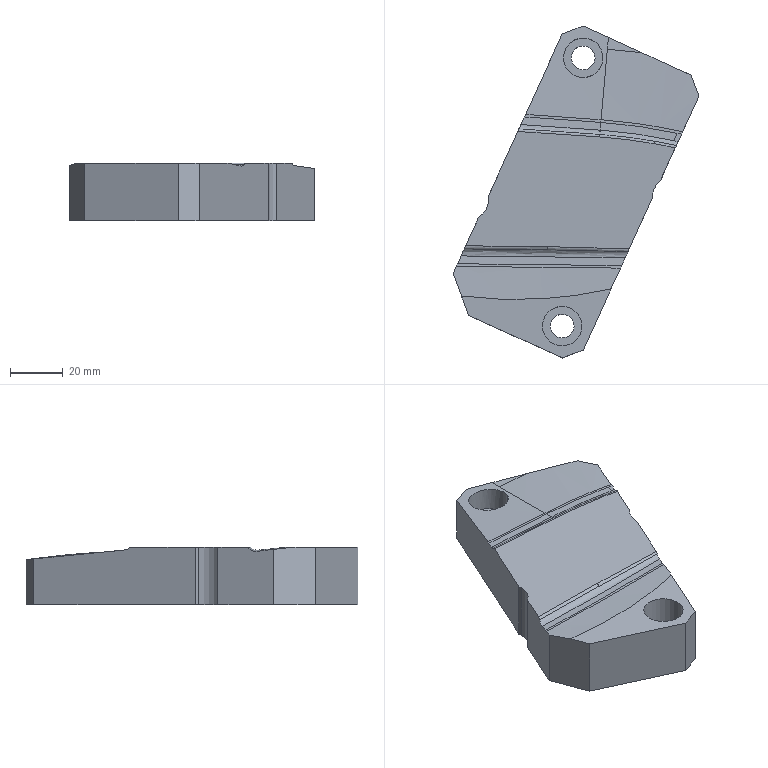Part | CATIA | 1 solid | 48 faces | box 93.337 x 126.037 x 22 mm | volume 134150 mm3 | spline 19 | plane 17 | cylinder 12 | commonest cylinder face diameters 9 x4 15 x4 18 x4